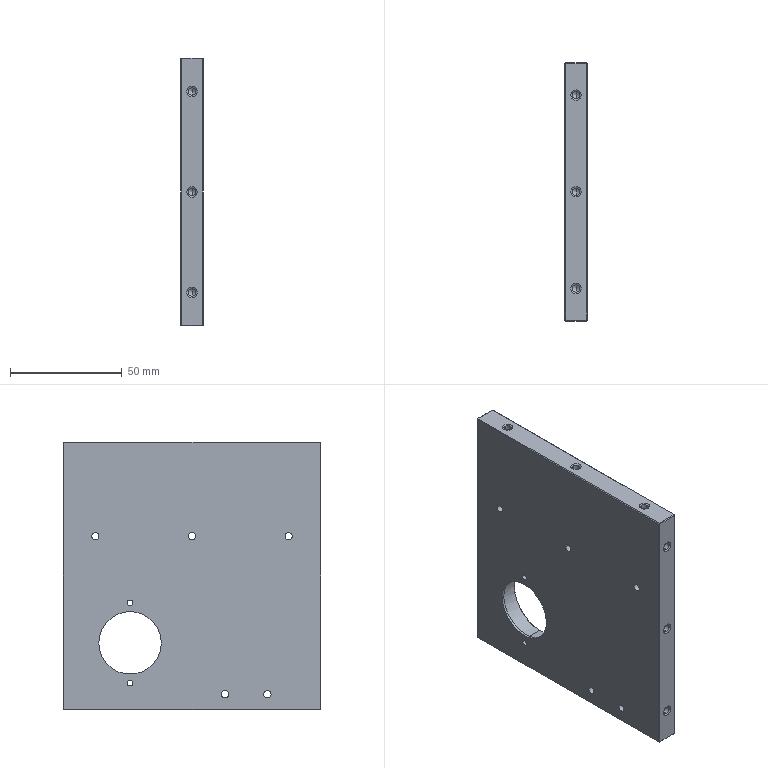Part | NX | 1 solid | 149 faces | box 10 x 115.5 x 120 mm | volume 128859 mm3 | cylinder 66 | cone 64 | plane 19 | commonest cylinder face diameters 3.3 x58 2.5 x4 28 x2 32 x2